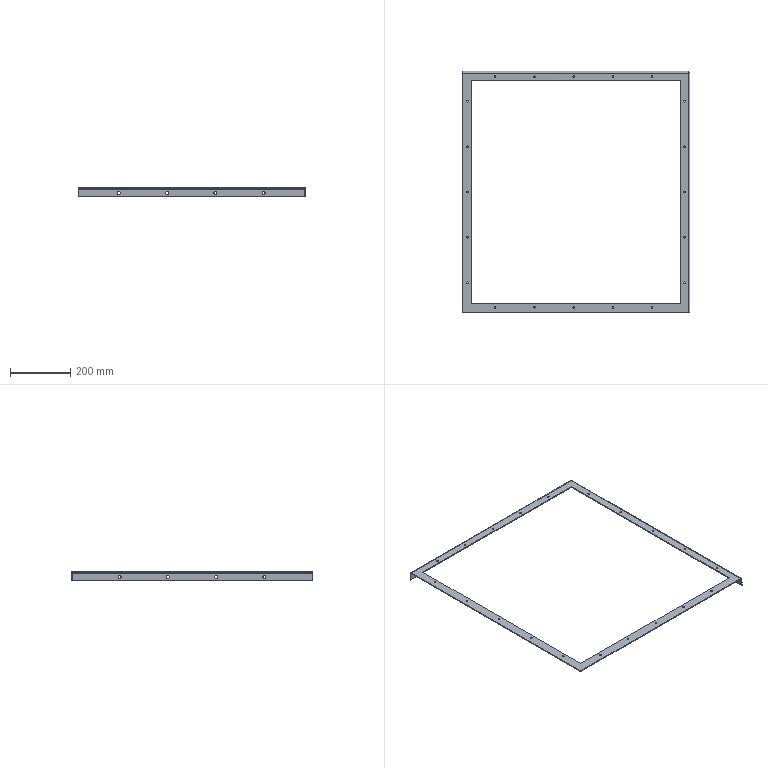Part | SolidWorks | features ICE 3, EdgeFlange 1, FlatPattern 1, SMBaseFlange 1, SheetMetal 1 | 1 solid | 82 faces | box 755 x 800 x 30 mm | volume 382350 mm3 | cylinder 60 | plane 20 | spline 2 | commonest cylinder face diameters 5 x40 10 x16 6 x2 12 x2